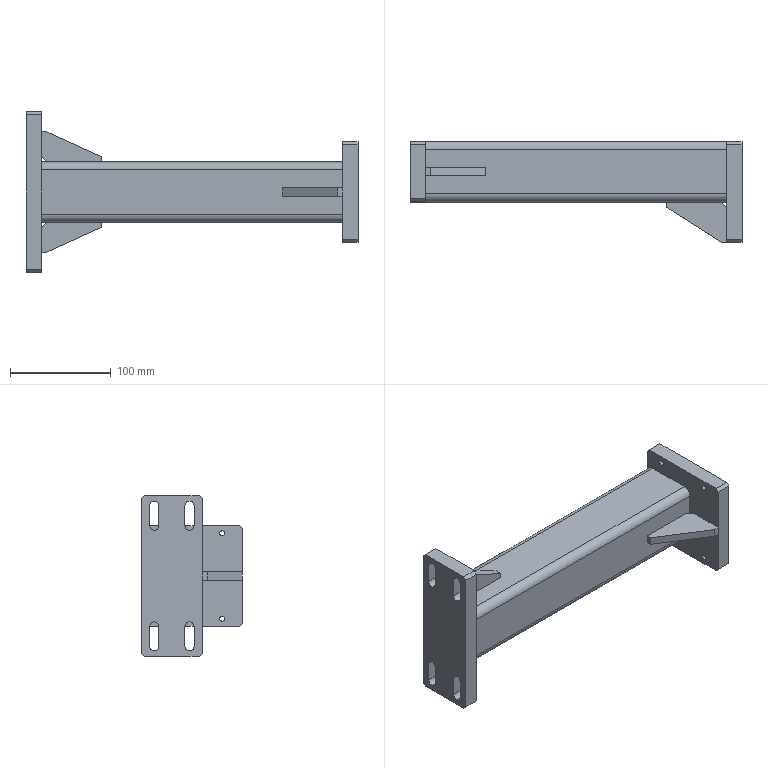Part | SolidWorks | features HoleWzd 4, ICE 4, Chamfer 2, MirrorSolid 1, WeldMemberFeat 1, WeldmentFeature 1 | 6 solids | 110 faces | box 330 x 100 x 160 mm | volume 561297 mm3 | plane 62 | cylinder 38 | cone 10 | commonest cylinder face diameters 5 x14 9 x12 6 x4 8 x4 16 x4